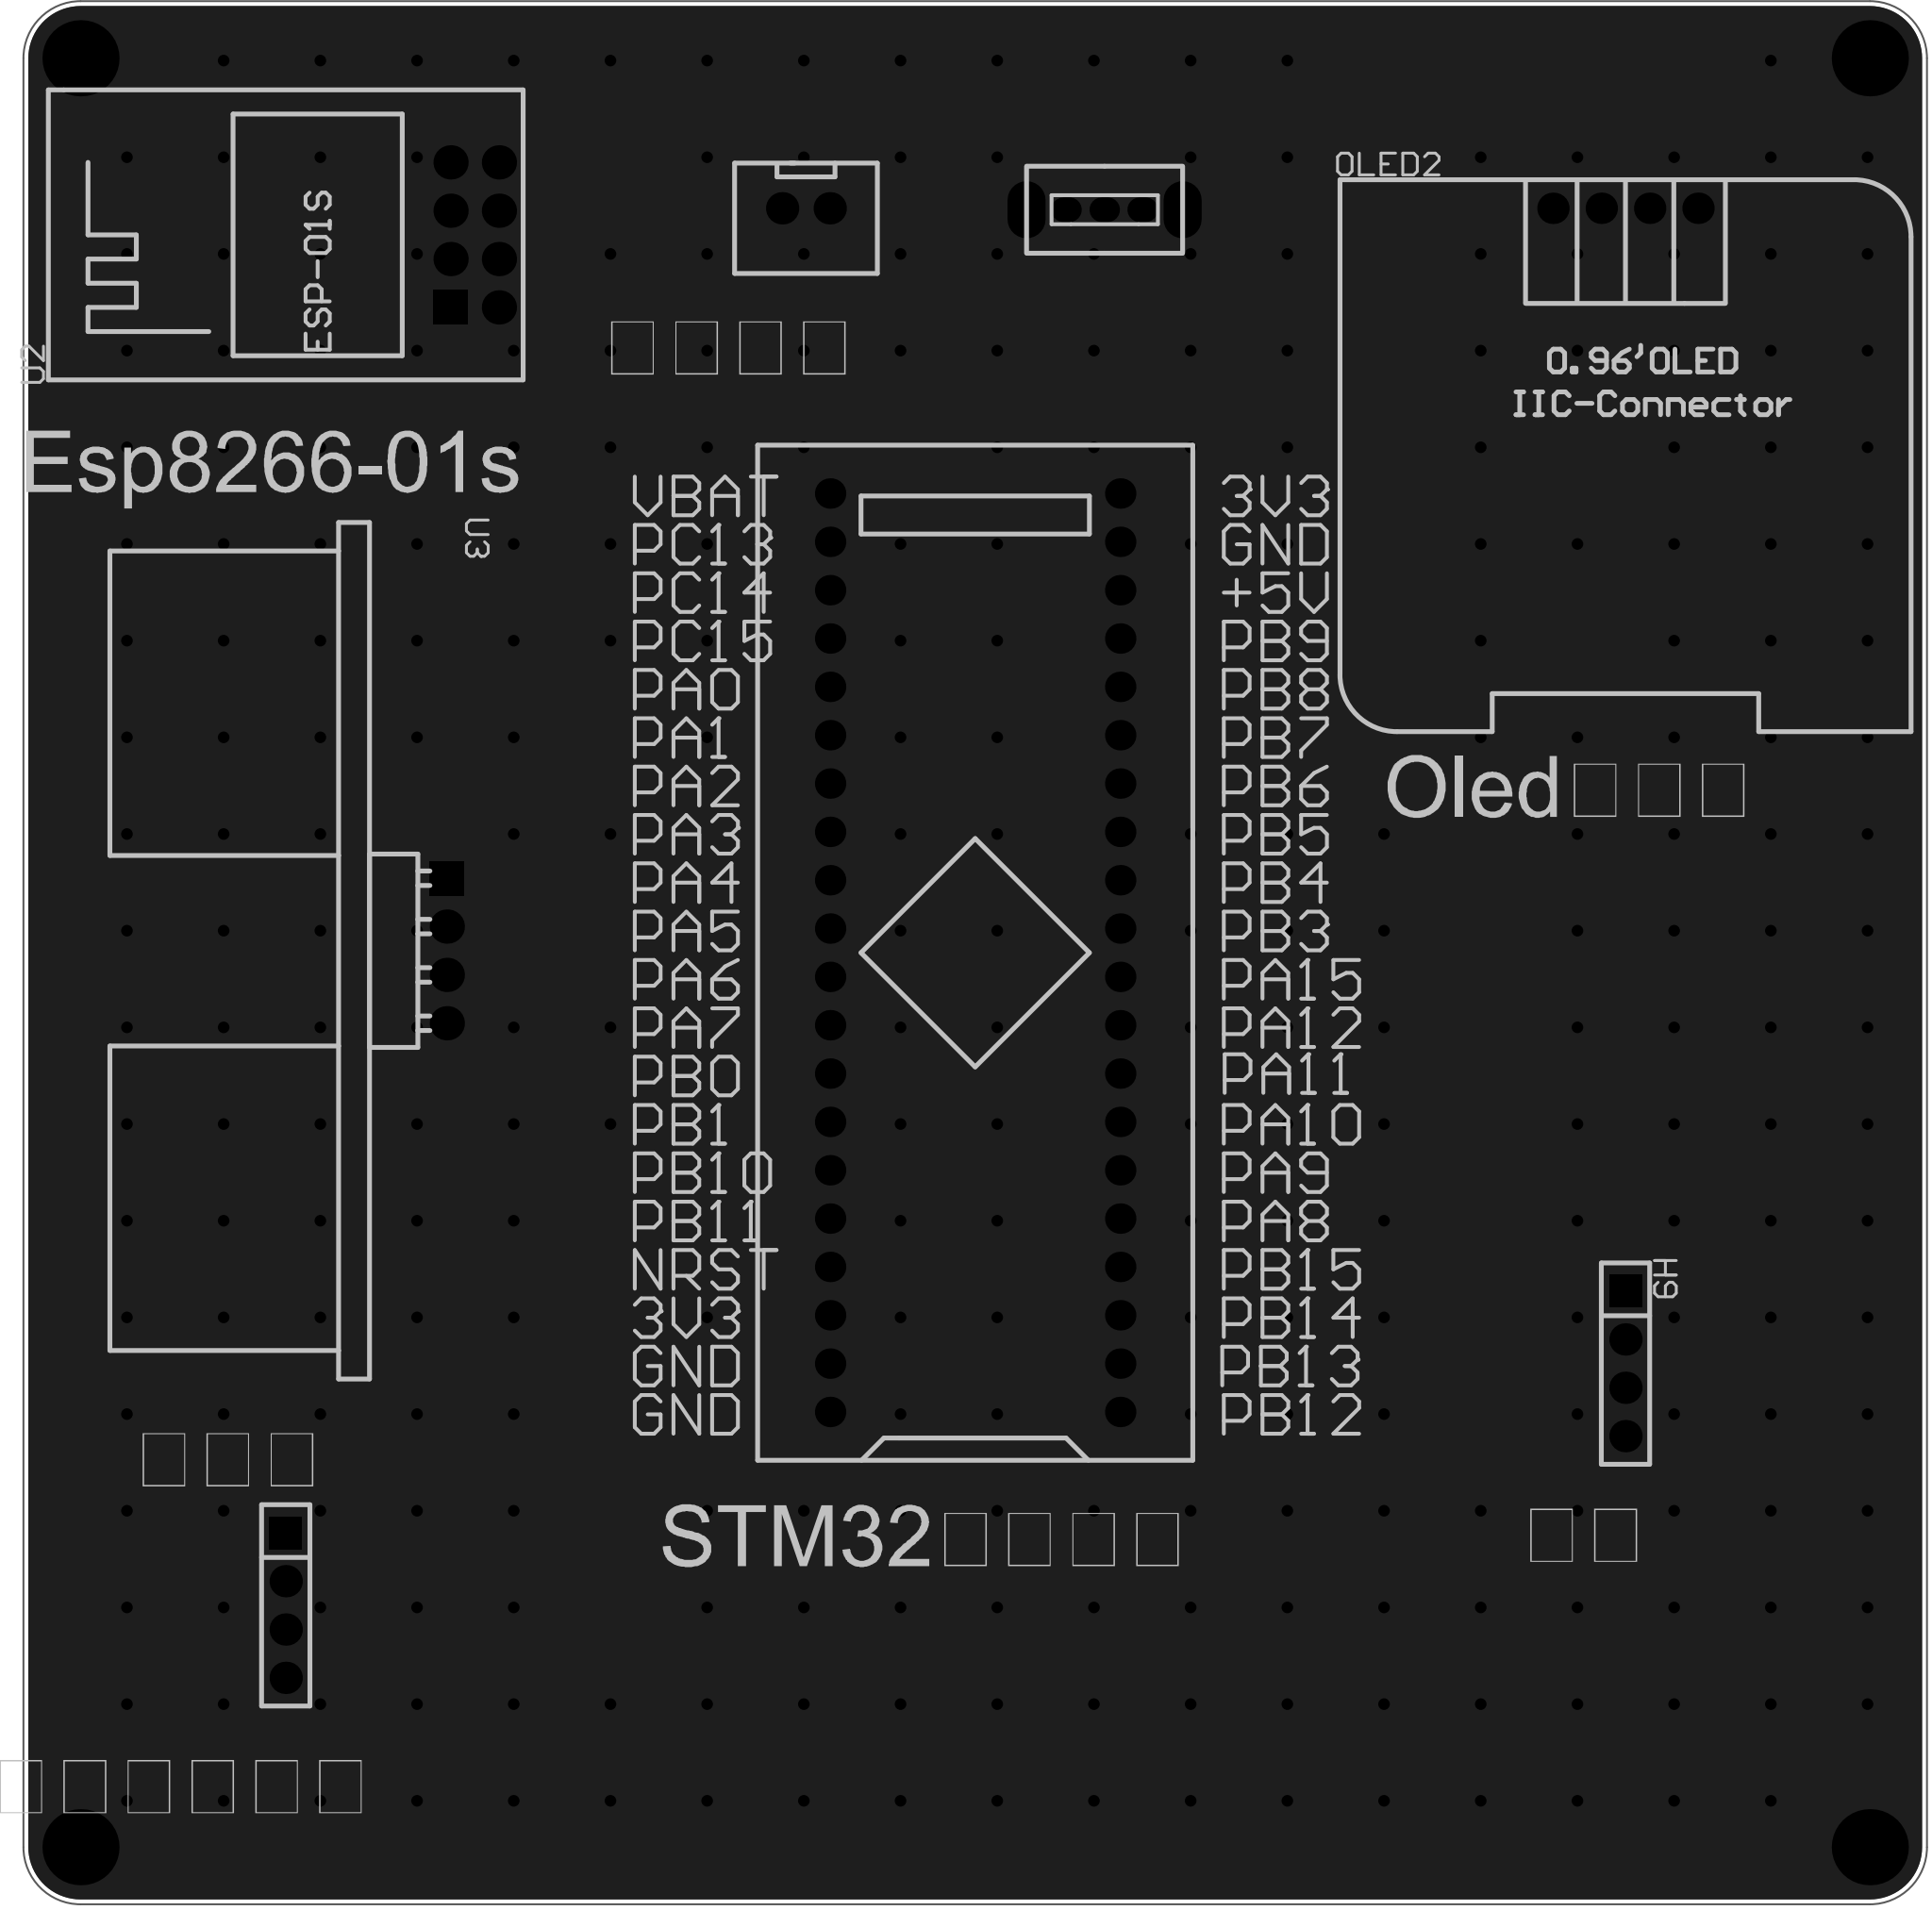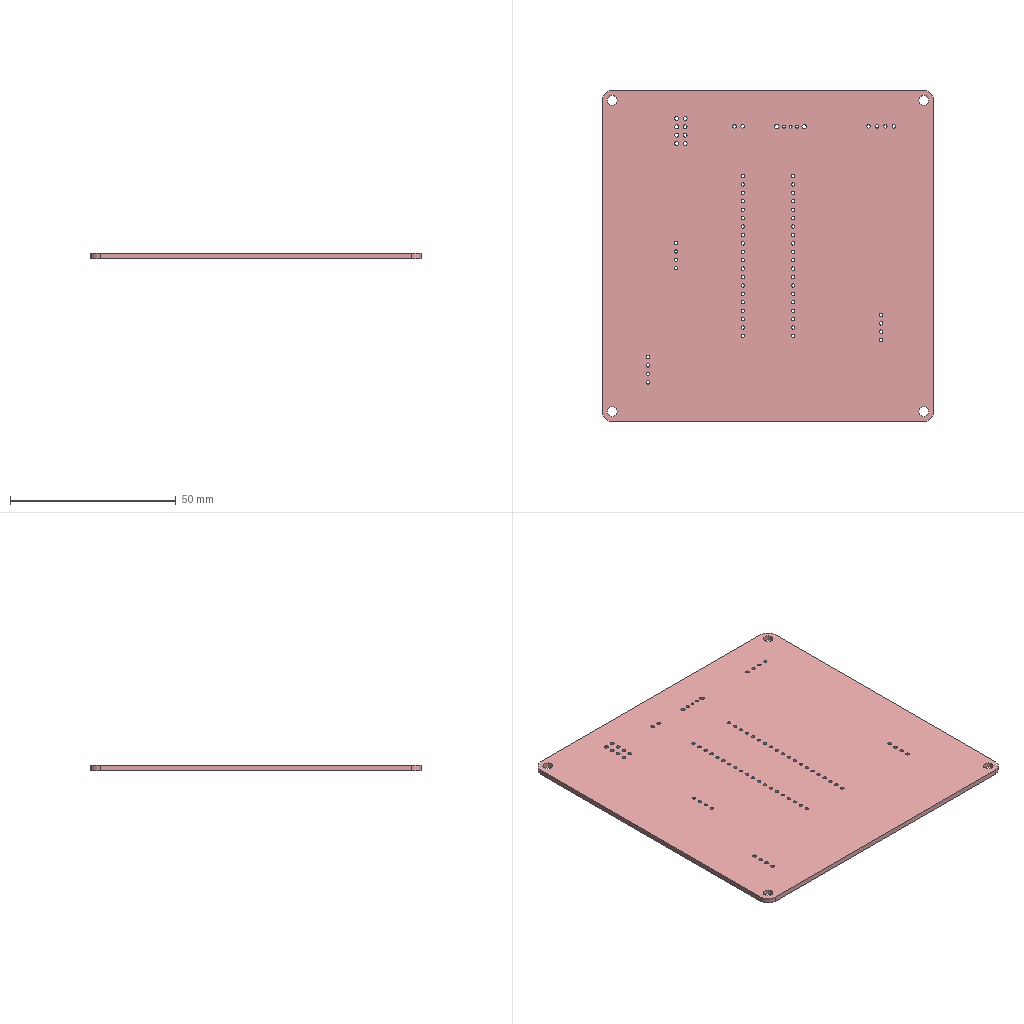Circuit board layout | Altium Designer | box 100 x 100 x 1.6 mm
Layer stack:
# Altium Designer layer stack of  (unit mm; dielectric type: 0 none, 1 core, 2 prepreg, 3 surface material)
index,name,kind,layer,copper_thickness_mm,dielectric_type,dielectric_thickness_mm,dielectric_material,dielectric_constant
0,Top Paste Mask Layer,other,,,,,,
1,Top Silkscreen Layer,other,,,,,,
2,Top Solder Mask Layer,dielectric,,,3,0.01,,3.3
3,Top Layer,copper,Top Layer,0.035,,,,
4,Dielectric1,dielectric,,,3,1.51,FR4,4.5
5,Bottom Layer,copper,Bottom Layer,0.035,,,,
6,Bottom Solder Mask Layer,dielectric,,,3,0.01,,3.3
7,Bottom Silkscreen Layer,other,,,,,,
8,Bottom Paste Mask Layer,other,,,,,,
# drill layer pairs: low layer,high layer
drill_pair,Top Layer,Bottom Layer
Part placement:
Designator,Comment,Layer,Footprint,Center-X(mm),Center-Y(mm),Rotation
U1,STM32F103C8T6-Card,TopLayer,CONN-TH_L53.3-W22.9_STM32F103C8T6-CARD,141.351,130.937,90
CN4,XH2.54*2P_直插,TopLayer,CONN-TH_2P-P2.50-XH2.54-2P,132.461,170.053,0
SW5,,TopLayer,拨动开关,148.148,169.978,180
H4,,TopLayer,HDR-TH_4P-P2.54-V-F,105.131,96.645,270
OLED2,,TopLayer,0.96OLED_4P,175.514,170.053,0
H9,,TopLayer,HDR-TH_4P-P2.54-V-F,175.514,109.347,270
U2,ESP-01S,TopLayer,WIFIM-TH_ESP-01S,115.062,168.656,90
U3,HC-SR04,TopLayer,TH_HC-SR04V,113.596,131.041,270
Pad and via stacks:
# Altium Designer via and pad stacks of  (unit mm). Each distinct definition once, with the count of objects using it.
# via: kind,start_layer,end_layer,hole_mm,diameter_mm,mode(0 simple;1 top-mid-bottom;2 full stack),diameter_per_layer,count,example_net
# pad: kind,layer,hole_mm,hole_type(0 round;1 square;2 slot),plating,top_size,top_shape(1 round;2 rect;3 octagon;9 rounded rect),mid_size,bottom_size,mode,footprint,size_per_layer,count,example
pad,Multi-Layer,3,0,plated,4x4,1,4x4,4x4,0,,,4,1
pad,Multi-Layer,1,0,plated,1.6x1.6,1,1.6x1.6,1.6x1.6,0,CONN-TH_L53.3-W22.9_STM32F103C8T6-CARD,,40,U1.1
pad,Multi-Layer,1.05,0,plated,1.7x1.7,1,1.7x1.7,1.7x1.7,0,CONN-TH_2P-P2.50-XH2.54-2P,,2,CN4.2
pad,Multi-Layer,0.8992,0,plated,1.6x1.3,1,1.6x1.3,1.6x1.3,0,\u00B2\u00A6\u00B6\u00AF\u00BF\u00AA\u00B9\u00D8,,3,SW5.1
pad,Multi-Layer,1.3,0,plated,3x1.999,1,3x1.999,3x1.999,0,\u00B2\u00A6\u00B6\u00AF\u00BF\u00AA\u00B9\u00D8,,2,SW5.4
pad,Multi-Layer,1.1,0,plated,1.7x1.7,2,1.7x1.7,1.7x1.7,0,HDR-TH_4P-P2.54-V-F,,2,H4.1
pad,Multi-Layer,1.1,0,plated,1.7x1.7,1,1.7x1.7,1.7x1.7,0,HDR-TH_4P-P2.54-V-F,,6,H4.2
pad,Multi-Layer,1,0,plated,1.65x1.65,1,1.65x1.65,1.65x1.65,0,0.96OLED_4P,,4,OLED2.4
pad,Multi-Layer,1.2,0,plated,1.8x1.8,2,1.8x1.8,1.8x1.8,0,WIFIM-TH_ESP-01S,,1,U2.1
pad,Multi-Layer,1.2,0,plated,1.8x1.8,1,1.8x1.8,1.8x1.8,0,WIFIM-TH_ESP-01S,,7,U2.2
pad,Multi-Layer,1.001,0,plated,1.8x1.8,1,1.8x1.8,1.8x1.8,0,TH_HC-SR04V,,3,U3.4
pad,Multi-Layer,1.001,0,plated,1.8x1.8,2,1.8x1.8,1.8x1.8,0,TH_HC-SR04V,,1,U3.1
via,Top Layer,Bottom Layer,0.3048,0.61,0,,294,GND
Copper pours:
name,layer,net,type(0 solid;1 hatched;2 none)
Bottom Layer-GND,Bottom Layer,GND,0
Top Layer-GND,Top Layer,GND,0
Design rules, without the lines most boards share:
# Altium Designer design rules of  (exported by Altium Designer, unit mm)
# columns: name | kind | enabled | priority | scope1 | scope2 | descriptor | typed fields (field=value)
Copper_copperRegion_copperThickness1oz | 0 | disabled | 4 | All | All | Clearance Constraint (Gap=5.984mil) (Disabled)(All),(All) | gap=0.152
Copper_copperRegion_copperThickness1oz_1 | 63 | disabled | 4 | All | All | Board Clearance Constraint (Gap=0mil) (Disabled)(All) |
Copper_copperRegion_Copper_copperRegion | 0 | disabled | 5 | All | All | Clearance Constraint (Gap=5.984mil) (Disabled)(All),(All) | gap=0.152
Copper_copperRegion_Copper_copperRegion_1 | 63 | disabled | 5 | All | All | Board Clearance Constraint (Gap=0mil) (Disabled)(All) |
copperThickness1oz | 0 | enabled | 6 | All | All | Clearance Constraint (Gap=5.984mil) (All),(All) | gap=0.152
copperThickness1oz_1 | 63 | enabled | 6 | All | All | Board Clearance Constraint (Gap=0mil) (All) |
copperRegion_copperThickness1oz | 20 | disabled | 1 | All | All | Polygon Connect Rule(Relief Connect )(Conductor Width=10mil) (Relief Angle=90 Angle) (Entries=4) (Air Gap Width=10mil) (Disabled)(All),(All) | connect_style(0=relief,1=direct,2=none)=0 relief_conductor_width=0.254 relief_entries=4
copperRegion_Copper_copperRegion | 20 | disabled | 2 | All | All | Polygon Connect Rule(Relief Connect )(Conductor Width=10mil) (Relief Angle=90 Angle) (Entries=4) (Air Gap Width=10mil) (Disabled)(All),(All) | connect_style(0=relief,1=direct,2=none)=0 relief_conductor_width=0.254 relief_entries=4
copperRegion | 20 | enabled | 3 | All | All | Polygon Connect Rule(Relief Connect )(Conductor Width=10mil) (Relief Angle=90 Angle) (Entries=4) (Air Gap Width=10mil) (All),(All) | connect_style(0=relief,1=direct,2=none)=0 relief_conductor_width=0.254 relief_entries=4